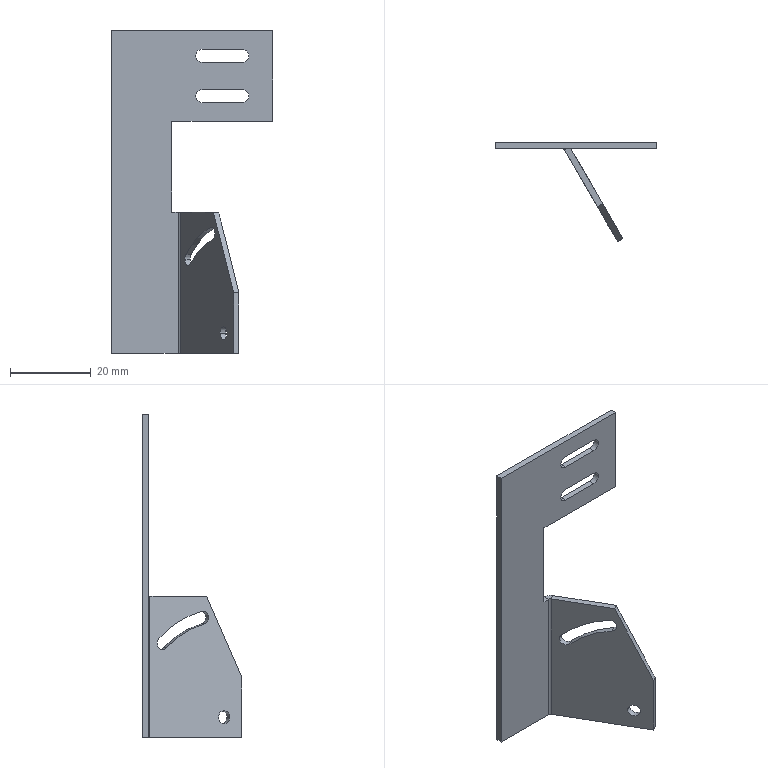Part | STEP file | PN_0010 | 1 solid | 34 faces | box 40 x 24.566 x 80 mm | volume 3826 mm3 | plane 21 | cylinder 13 | commonest cylinder face diameters 3.2 x9 1.473 x1 4.473 x1 47.6 x1 54 x1